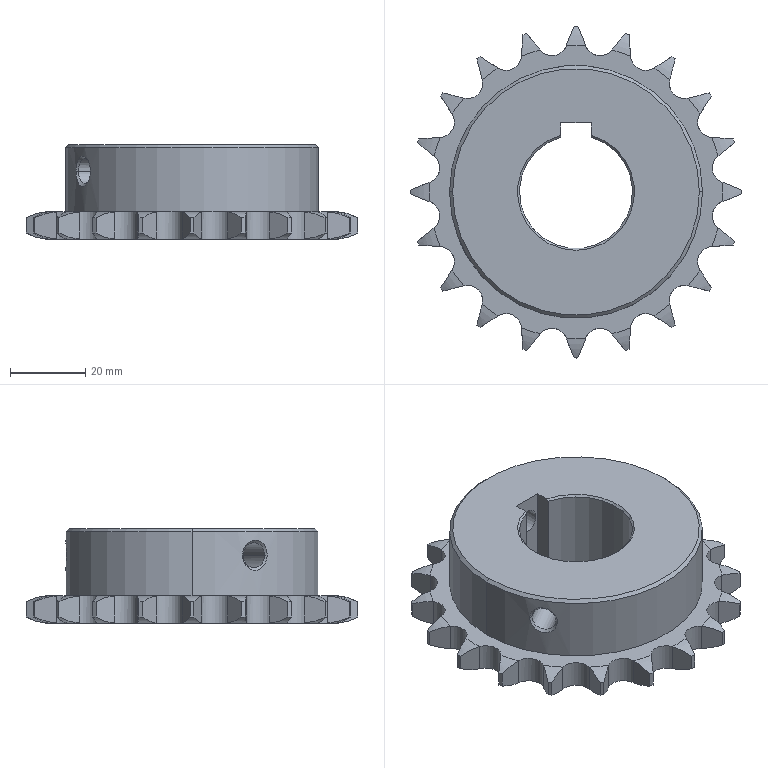Part | SolidWorks | features BaseBody 1 | 1 solid | 123 faces | box 88 x 88 x 25.063 mm | volume 77723 mm3 | cylinder 47 | plane 46 | torus 22 | cone 8 | commonest cylinder face diameters 8.04 x20 88 x20 6.647 x4 67 x2 30 x1